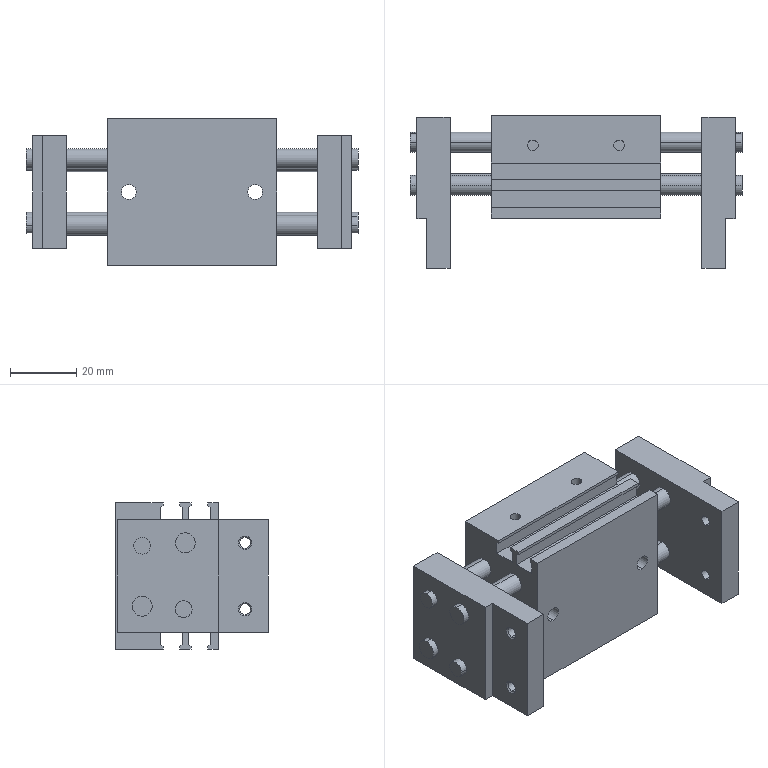Part | SolidWorks | 7 solids | 178 faces | box 100 x 46 x 44 mm | volume 92553 mm3 | plane 79 | cylinder 75 | cone 24 | commonest cylinder face diameters 6 x24 3.242 x20 4.134 x12 5 x8 3 x5 4.5 x4